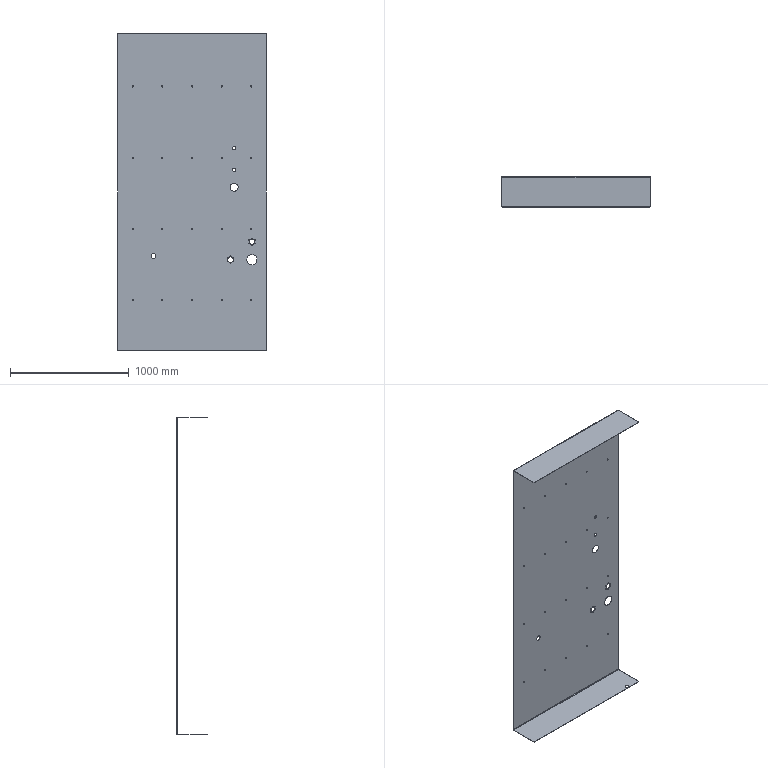Part | STEP file | VD-SYL0380DJ1006_1_2_1-2_STEP | 1 solid | 106 faces | box 1250 x 254 x 2680 mm | volume 11864231 mm3 | cylinder 84 | plane 22 | commonest cylinder face diameters 10 x40 4.2 x24 48 x4 6 x2 12 x2 27 x2